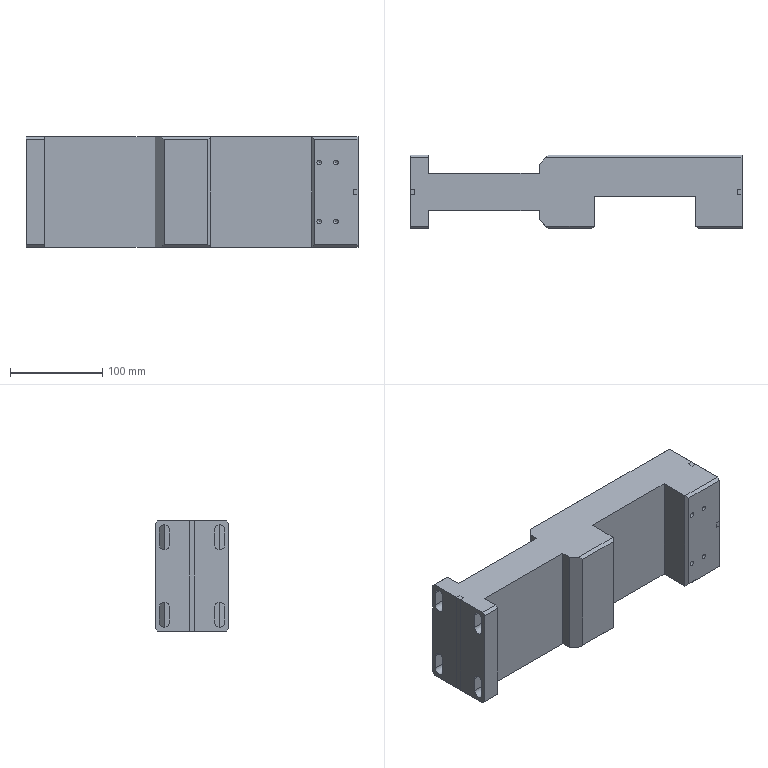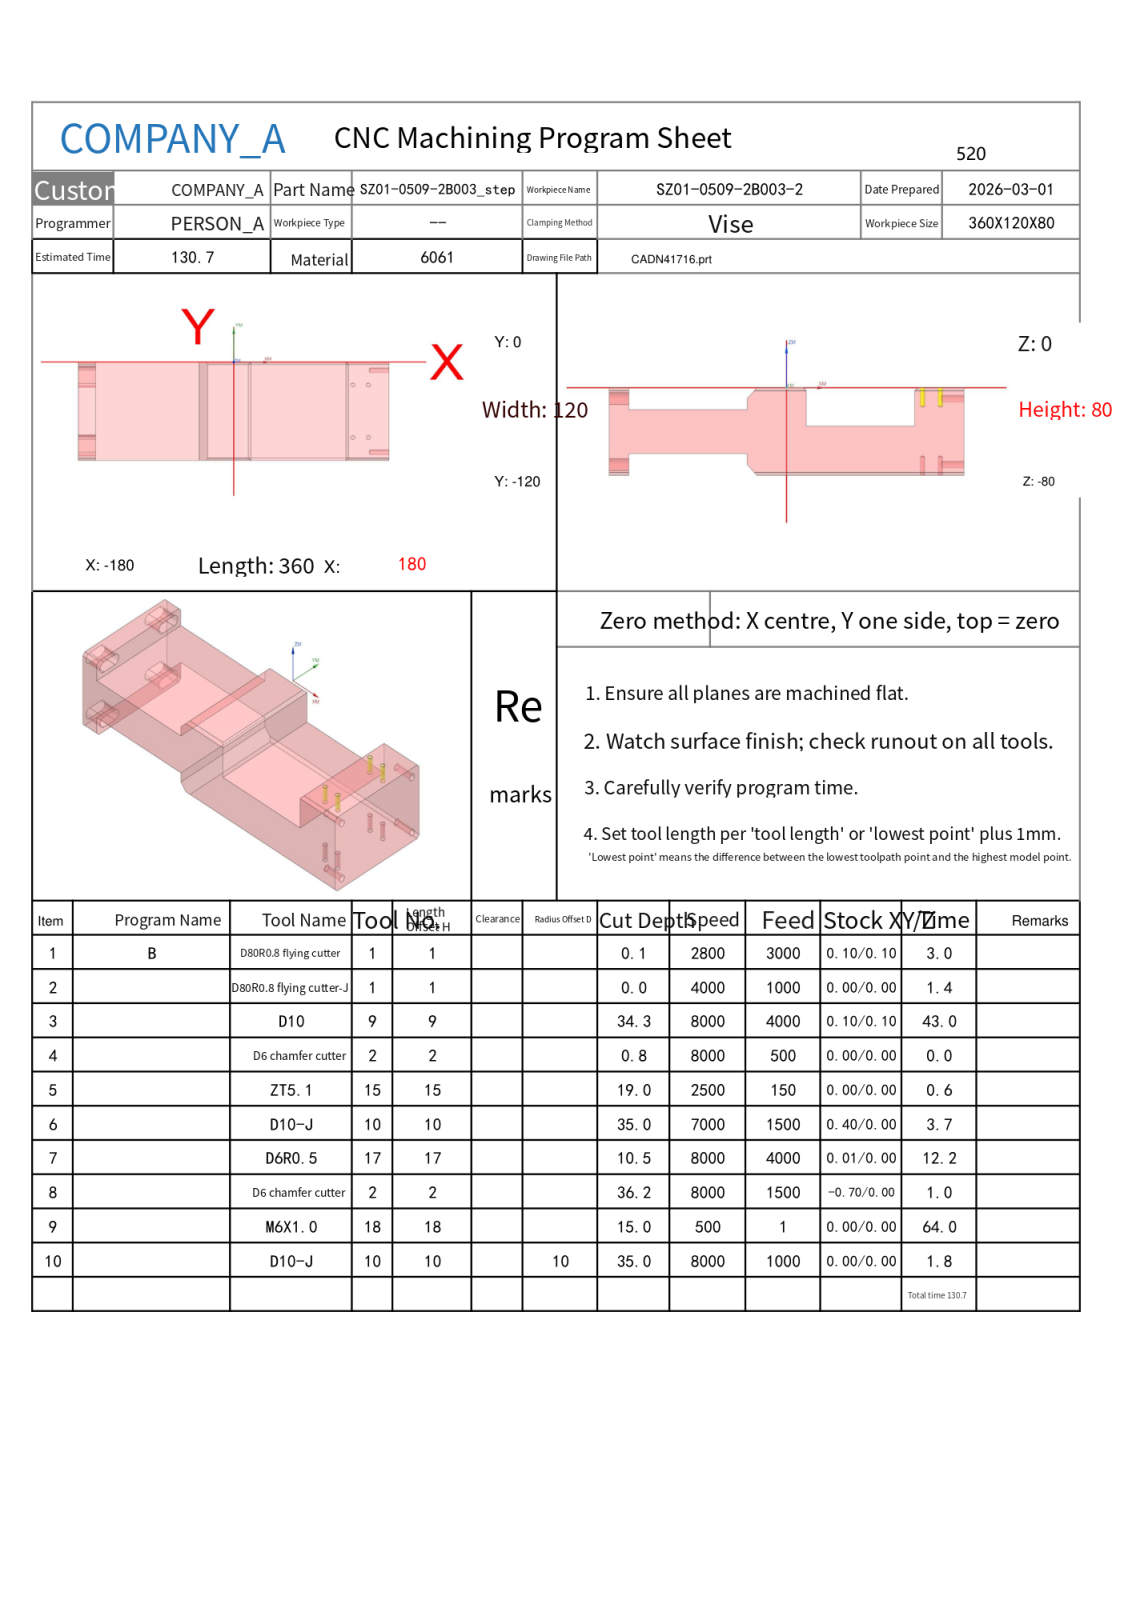NC program | NX | posted by the shop | part box 360 x 80 x 120 mm
Lines 1 to 150 of 12457:
%
O0001
(Machine time: 192.59 MIN)
(===Total Tool:7===)
(T1=D80R0.8 flying cutter D=80.  R=0.8  D-  H01 Z=0.    )
(T9=D10     D=10.  R=0.   D-  H09 Z=-34.31)
(T2=D6 chamfer cutter   D=6.   R=0.   D-  H02 Z=-36.2 )
(T15=ZT5.1  D=5.1  DR_a=118 D-  H15 Z=-19.  )
(T10=D10-J  D=10.  R=0.   D-  H10 Z=-35.  )
(T17=D6R0.5 D=6.   R=0.5  D-  H17 Z=-10.5 )
(T18=M6X1.0 D=5.   DR_a=180 D-  H18 Z=-15.  )
G80 G90 G17 G49 G40
G91 G28 Z0
M01
N1 T01 M06
(D80R0.8 flying cutter  D=80. R=0.8 H=01 ce=0.10 di=0.10)
G00 G90 G54 X232.097 Y-96.097 M03 S2800
G43 H01 Z50.
M08
Z6.011
G01 Z4.011 F3000.
X220.097
X-212.101
G02 X-220.097 Y-88.1 I.004 J8.
G01 Y-39.259
G02 X-212.101 Y-31.263 I8. J-.004
G01 X220.097
X232.097
Z6.011
G00 Y-96.097
Z5.522
G01 Z3.522
X220.097
X-212.101
G02 X-220.097 Y-88.1 I.004 J8.
G01 Y-39.259
G02 X-212.101 Y-31.263 I8. J-.004
G01 X220.097
X232.097
Z5.522
G00 Y-96.097
Z5.033
G01 Z3.033
X220.097
X-212.101
G02 X-220.097 Y-88.1 I.004 J8.
G01 Y-39.259
G02 X-212.101 Y-31.263 I8. J-.004
G01 X220.097
X232.097
Z5.033
G00 Y-96.097
Z4.544
G01 Z2.544
X220.097
X-212.101
G02 X-220.097 Y-88.1 I.004 J8.
G01 Y-39.259
G02 X-212.101 Y-31.263 I8. J-.004
G01 X220.097
X232.097
Z4.544
G00 Y-96.097
Z4.056
G01 Z2.056
X220.097
X-212.101
G02 X-220.097 Y-88.1 I.004 J8.
G01 Y-39.259
G02 X-212.101 Y-31.263 I8. J-.004
G01 X220.097
X232.097
Z4.056
G00 Y-96.097
Z3.567
G01 Z1.567
X220.097
X-212.101
G02 X-220.097 Y-88.1 I.004 J8.
G01 Y-39.259
G02 X-212.101 Y-31.263 I8. J-.004
G01 X220.097
X232.097
Z3.567
G00 Y-96.097
Z3.078
G01 Z1.078
X220.097
X-212.101
G02 X-220.097 Y-88.1 I.004 J8.
G01 Y-39.259
G02 X-212.101 Y-31.263 I8. J-.004
G01 X220.097
X232.097
Z3.078
G00 Y-96.097
Z2.589
G01 Z.589
X220.097
X-212.101
G02 X-220.097 Y-88.1 I.004 J8.
G01 Y-39.259
G02 X-212.101 Y-31.263 I8. J-.004
G01 X220.097
X232.097
Z2.589
G00 Y-96.097
Z2.1
G01 Z.1
X220.097
X-212.101
G02 X-220.097 Y-88.1 I.004 J8.
G01 Y-39.259
G02 X-212.101 Y-31.263 I8. J-.004
G01 X220.097
X232.097
Z2.1
G00 Z50.
G91 G28 Z0.0
M05
M09
G91 G28 Z0.0
M01
N2 T01 M06
(D80R0.8 flying cutter-J  D=80. R=0.8 H=01 ce=0.00 di=0.00)
G00 G90 G54 X231.999 Y-95.999 M03 S4000
G43 H01 Z50.
M08
Z2.
G01 Z0.0 F1000.
X219.999
X-212.799
G02 X-219.999 Y-88.799 I0.0 J7.2
G01 Y-71.68
G02 X-211.999 Y-63.68 I8. J0.0
G01 X212.799
G03 X219.999 Y-56.48 I0.0 J7.2
G01 Y-39.361
G03 X211.999 Y-31.361 I-8. J0.0
G01 X-219.999
X-231.999
Z2.
G00 Z50.
G91 G28 Z0.0
M05
M09
G91 G28 Z0.0
M01